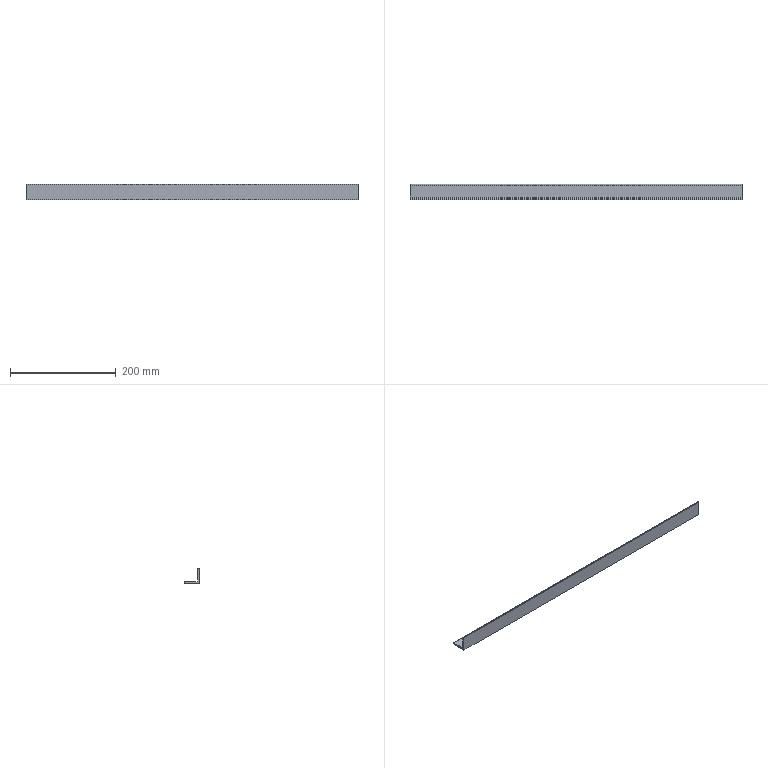Part | NX | features BREP 1 | 1 solid | 11 faces | box 627.062 x 28.575 x 28.575 mm | volume 107121 mm3 | plane 8 | cylinder 3 | commonest cylinder face diameters 3.175 x3
STEP:
#1=CARTESIAN_POINT('',(-313.531,-1.587,25.4));
#2=VERTEX_POINT('',#1);
#3=CARTESIAN_POINT('',(-313.531,0.,23.812));
#4=VERTEX_POINT('',#3);
#5=CARTESIAN_POINT('',(-313.531,-1.587,23.812));
#6=DIRECTION('',(-1.,0.,0.));
#7=DIRECTION('',(0.,0.,1.));
#8=AXIS2_PLACEMENT_3D('',#5,#6,#7);
#9=CIRCLE('',#8,1.587);
#10=EDGE_CURVE('',#2,#4,#9,.T.);
#11=ORIENTED_EDGE('',*,*,#10,.T.);
#12=CARTESIAN_POINT('',(-313.531,0.,1.587));
#13=VERTEX_POINT('',#12);
#14=CARTESIAN_POINT('',(-313.531,0.,1.587));
#15=DIRECTION('',(0.,0.,1.));
#16=VECTOR('',#15,1000.);
#17=LINE('',#14,#16);
#18=EDGE_CURVE('',#13,#4,#17,.T.);
#19=ORIENTED_EDGE('',*,*,#18,.F.);
#20=CARTESIAN_POINT('',(-313.531,1.587,0.));
#21=VERTEX_POINT('',#20);
#22=CARTESIAN_POINT('',(-313.531,1.587,1.587));
#23=DIRECTION('',(1.,0.,0.));
#24=DIRECTION('',(0.,-1.,0.));
#25=AXIS2_PLACEMENT_3D('',#22,#23,#24);
#26=CIRCLE('',#25,1.587);
#27=EDGE_CURVE('',#13,#21,#26,.T.);
#28=ORIENTED_EDGE('',*,*,#27,.T.);
#29=CARTESIAN_POINT('',(-313.531,23.812,0.));
#30=VERTEX_POINT('',#29);
#31=CARTESIAN_POINT('',(-313.531,23.812,0.));
#32=DIRECTION('',(0.,-1.,0.));
#33=VECTOR('',#32,1000.);
#34=LINE('',#31,#33);
#35=EDGE_CURVE('',#30,#21,#34,.T.);
#36=ORIENTED_EDGE('',*,*,#35,.F.);
#37=CARTESIAN_POINT('',(-313.531,25.4,-1.587));
#38=VERTEX_POINT('',#37);
#39=CARTESIAN_POINT('',(-313.531,23.812,-1.587));
#40=DIRECTION('',(-1.,0.,0.));
#41=DIRECTION('',(0.,0.,1.));
#42=AXIS2_PLACEMENT_3D('',#39,#40,#41);
#43=CIRCLE('',#42,1.587);
#44=EDGE_CURVE('',#30,#38,#43,.T.);
#45=ORIENTED_EDGE('',*,*,#44,.T.);
#46=CARTESIAN_POINT('',(-313.531,25.4,-3.175));
#47=VERTEX_POINT('',#46);
#48=CARTESIAN_POINT('',(-313.531,25.4,-3.175));
#49=DIRECTION('',(0.,0.,1.));
#50=VECTOR('',#49,1000.);
#51=LINE('',#48,#50);
#52=EDGE_CURVE('',#47,#38,#51,.T.);
#53=ORIENTED_EDGE('',*,*,#52,.F.);
#54=CARTESIAN_POINT('',(-313.531,-3.175,-3.175));
#55=VERTEX_POINT('',#54);
#56=CARTESIAN_POINT('',(-313.531,-3.175,-3.175));
#57=DIRECTION('',(0.,1.,0.));
#58=VECTOR('',#57,1000.);
#59=LINE('',#56,#58);
#60=EDGE_CURVE('',#55,#47,#59,.T.);
#61=ORIENTED_EDGE('',*,*,#60,.F.);
#62=CARTESIAN_POINT('',(-313.531,-3.175,25.4));
#63=VERTEX_POINT('',#62);
#64=CARTESIAN_POINT('',(-313.531,-3.175,25.4));
#65=DIRECTION('',(0.,0.,-1.));
#66=VECTOR('',#65,1000.);
#67=LINE('',#64,#66);
#68=EDGE_CURVE('',#63,#55,#67,.T.);
#69=ORIENTED_EDGE('',*,*,#68,.F.);
#70=CARTESIAN_POINT('',(-313.531,-1.587,25.4));
#71=DIRECTION('',(0.,-1.,0.));
#72=VECTOR('',#71,1000.);
#73=LINE('',#70,#72);
#74=EDGE_CURVE('',#2,#63,#73,.T.);
#75=ORIENTED_EDGE('',*,*,#74,.F.);
#76=EDGE_LOOP('',(#11,#19,#28,#36,#45,#53,#61,#69,#75));
#77=FACE_BOUND('',#76,.T.);
#78=CARTESIAN_POINT('',(-313.531,0.,0.));
#79=DIRECTION('',(1.,0.,0.));
#80=DIRECTION('',(0.,1.,0.));
#81=AXIS2_PLACEMENT_3D('',#78,#79,#80);
#82=PLANE('',#81);
#83=ADVANCED_FACE('',(#77),#82,.F.);
#84=CARTESIAN_POINT('',(313.531,-3.175,25.4));
#85=VERTEX_POINT('',#84);
#86=CARTESIAN_POINT('',(-313.531,-3.175,25.4));
#87=DIRECTION('',(1.,0.,0.));
#88=VECTOR('',#87,1000.);
#89=LINE('',#86,#88);
#90=EDGE_CURVE('',#63,#85,#89,.T.);
#91=ORIENTED_EDGE('',*,*,#90,.T.);
#92=CARTESIAN_POINT('',(313.531,-1.587,25.4));
#93=VERTEX_POINT('',#92);
#94=CARTESIAN_POINT('',(313.531,-1.587,25.4));
#95=DIRECTION('',(0.,-1.,0.));
#96=VECTOR('',#95,1000.);
#97=LINE('',#94,#96);
#98=EDGE_CURVE('',#93,#85,#97,.T.);
#99=ORIENTED_EDGE('',*,*,#98,.F.);
#100=CARTESIAN_POINT('',(313.531,-1.587,25.4));
#101=DIRECTION('',(-1.,0.,0.));
#102=VECTOR('',#101,1000.);
#103=LINE('',#100,#102);
#104=EDGE_CURVE('',#93,#2,#103,.T.);
#105=ORIENTED_EDGE('',*,*,#104,.T.);
#106=ORIENTED_EDGE('',*,*,#74,.T.);
#107=EDGE_LOOP('',(#91,#99,#105,#106));
#108=FACE_BOUND('',#107,.T.);
#109=CARTESIAN_POINT('',(-313.531,0.,25.4));
#110=DIRECTION('',(0.,0.,1.));
#111=DIRECTION('',(1.,0.,0.));
#112=AXIS2_PLACEMENT_3D('',#109,#110,#111);
#113=PLANE('',#112);
#114=ADVANCED_FACE('',(#108),#113,.T.);
#115=CARTESIAN_POINT('',(313.531,0.,23.812));
#116=VERTEX_POINT('',#115);
#117=CARTESIAN_POINT('',(313.531,-1.587,23.812));
#118=DIRECTION('',(1.,0.,0.));
#119=DIRECTION('',(0.,1.,0.));
#120=AXIS2_PLACEMENT_3D('',#117,#118,#119);
#121=CIRCLE('',#120,1.587);
#122=EDGE_CURVE('',#116,#93,#121,.T.);
#123=ORIENTED_EDGE('',*,*,#122,.F.);
#124=CARTESIAN_POINT('',(313.531,0.,23.812));
#125=DIRECTION('',(-1.,0.,0.));
#126=VECTOR('',#125,1000.);
#127=LINE('',#124,#126);
#128=EDGE_CURVE('',#116,#4,#127,.T.);
#129=ORIENTED_EDGE('',*,*,#128,.T.);
#130=ORIENTED_EDGE('',*,*,#10,.F.);
#131=ORIENTED_EDGE('',*,*,#104,.F.);
#132=EDGE_LOOP('',(#123,#129,#130,#131));
#133=FACE_BOUND('',#132,.T.);
#134=CARTESIAN_POINT('',(314.514,-1.587,23.812));
#135=DIRECTION('',(-1.,0.,0.));
#136=DIRECTION('',(0.,0.,1.));
#137=AXIS2_PLACEMENT_3D('',#134,#135,#136);
#138=CYLINDRICAL_SURFACE('',#137,1.587);
#139=ADVANCED_FACE('',(#133),#138,.T.);
#140=CARTESIAN_POINT('',(313.531,0.,1.587));
#141=VERTEX_POINT('',#140);
#142=CARTESIAN_POINT('',(313.531,0.,1.587));
#143=DIRECTION('',(0.,0.,1.));
#144=VECTOR('',#143,1000.);
#145=LINE('',#142,#144);
#146=EDGE_CURVE('',#141,#116,#145,.T.);
#147=ORIENTED_EDGE('',*,*,#146,.F.);
#148=CARTESIAN_POINT('',(-313.531,0.,1.587));
#149=DIRECTION('',(1.,0.,0.));
#150=VECTOR('',#149,1000.);
#151=LINE('',#148,#150);
#152=EDGE_CURVE('',#13,#141,#151,.T.);
#153=ORIENTED_EDGE('',*,*,#152,.F.);
#154=ORIENTED_EDGE('',*,*,#18,.T.);
#155=ORIENTED_EDGE('',*,*,#128,.F.);
#156=EDGE_LOOP('',(#147,#153,#154,#155));
#157=FACE_BOUND('',#156,.T.);
#158=CARTESIAN_POINT('',(-313.531,0.,0.));
#159=DIRECTION('',(0.,1.,0.));
#160=DIRECTION('',(1.,0.,0.));
#161=AXIS2_PLACEMENT_3D('',#158,#159,#160);
#162=PLANE('',#161);
#163=ADVANCED_FACE('',(#157),#162,.T.);
#164=CARTESIAN_POINT('',(313.531,1.587,0.));
#165=VERTEX_POINT('',#164);
#166=CARTESIAN_POINT('',(313.531,1.587,1.587));
#167=DIRECTION('',(-1.,0.,0.));
#168=DIRECTION('',(0.,0.,-1.));
#169=AXIS2_PLACEMENT_3D('',#166,#167,#168);
#170=CIRCLE('',#169,1.587);
#171=EDGE_CURVE('',#165,#141,#170,.T.);
#172=ORIENTED_EDGE('',*,*,#171,.F.);
#173=CARTESIAN_POINT('',(-313.531,1.587,0.));
#174=DIRECTION('',(1.,0.,0.));
#175=VECTOR('',#174,1000.);
#176=LINE('',#173,#175);
#177=EDGE_CURVE('',#21,#165,#176,.T.);
#178=ORIENTED_EDGE('',*,*,#177,.F.);
#179=ORIENTED_EDGE('',*,*,#27,.F.);
#180=ORIENTED_EDGE('',*,*,#152,.T.);
#181=EDGE_LOOP('',(#172,#178,#179,#180));
#182=FACE_BOUND('',#181,.T.);
#183=CARTESIAN_POINT('',(-314.371,1.587,1.587));
#184=DIRECTION('',(1.,0.,0.));
#185=DIRECTION('',(0.,-1.,0.));
#186=AXIS2_PLACEMENT_3D('',#183,#184,#185);
#187=CYLINDRICAL_SURFACE('',#186,1.587);
#188=ADVANCED_FACE('',(#182),#187,.F.);
#189=ORIENTED_EDGE('',*,*,#35,.T.);
#190=ORIENTED_EDGE('',*,*,#177,.T.);
#191=CARTESIAN_POINT('',(313.531,23.812,0.));
#192=VERTEX_POINT('',#191);
#193=CARTESIAN_POINT('',(313.531,23.812,0.));
#194=DIRECTION('',(0.,-1.,0.));
#195=VECTOR('',#194,1000.);
#196=LINE('',#193,#195);
#197=EDGE_CURVE('',#192,#165,#196,.T.);
#198=ORIENTED_EDGE('',*,*,#197,.F.);
#199=CARTESIAN_POINT('',(313.531,23.812,0.));
#200=DIRECTION('',(-1.,0.,0.));
#201=VECTOR('',#200,1000.);
#202=LINE('',#199,#201);
#203=EDGE_CURVE('',#192,#30,#202,.T.);
#204=ORIENTED_EDGE('',*,*,#203,.T.);
#205=EDGE_LOOP('',(#189,#190,#198,#204));
#206=FACE_BOUND('',#205,.T.);
#207=CARTESIAN_POINT('',(-313.531,25.4,0.));
#208=DIRECTION('',(0.,0.,1.));
#209=DIRECTION('',(1.,0.,0.));
#210=AXIS2_PLACEMENT_3D('',#207,#208,#209);
#211=PLANE('',#210);
#212=ADVANCED_FACE('',(#206),#211,.T.);
#213=CARTESIAN_POINT('',(313.531,25.4,-1.587));
#214=VERTEX_POINT('',#213);
#215=CARTESIAN_POINT('',(313.531,23.812,-1.587));
#216=DIRECTION('',(1.,0.,0.));
#217=DIRECTION('',(0.,1.,0.));
#218=AXIS2_PLACEMENT_3D('',#215,#216,#217);
#219=CIRCLE('',#218,1.587);
#220=EDGE_CURVE('',#214,#192,#219,.T.);
#221=ORIENTED_EDGE('',*,*,#220,.F.);
#222=CARTESIAN_POINT('',(313.531,25.4,-1.587));
#223=DIRECTION('',(-1.,0.,0.));
#224=VECTOR('',#223,1000.);
#225=LINE('',#222,#224);
#226=EDGE_CURVE('',#214,#38,#225,.T.);
#227=ORIENTED_EDGE('',*,*,#226,.T.);
#228=ORIENTED_EDGE('',*,*,#44,.F.);
#229=ORIENTED_EDGE('',*,*,#203,.F.);
#230=EDGE_LOOP('',(#221,#227,#228,#229));
#231=FACE_BOUND('',#230,.T.);
#232=CARTESIAN_POINT('',(314.514,23.812,-1.587));
#233=DIRECTION('',(-1.,0.,0.));
#234=DIRECTION('',(0.,0.,1.));
#235=AXIS2_PLACEMENT_3D('',#232,#233,#234);
#236=CYLINDRICAL_SURFACE('',#235,1.587);
#237=ADVANCED_FACE('',(#231),#236,.T.);
#238=ORIENTED_EDGE('',*,*,#226,.F.);
#239=CARTESIAN_POINT('',(313.531,25.4,-3.175));
#240=VERTEX_POINT('',#239);
#241=CARTESIAN_POINT('',(313.531,25.4,-3.175));
#242=DIRECTION('',(0.,0.,1.));
#243=VECTOR('',#242,1000.);
#244=LINE('',#241,#243);
#245=EDGE_CURVE('',#240,#214,#244,.T.);
#246=ORIENTED_EDGE('',*,*,#245,.F.);
#247=CARTESIAN_POINT('',(-313.531,25.4,-3.175));
#248=DIRECTION('',(1.,0.,0.));
#249=VECTOR('',#248,1000.);
#250=LINE('',#247,#249);
#251=EDGE_CURVE('',#47,#240,#250,.T.);
#252=ORIENTED_EDGE('',*,*,#251,.F.);
#253=ORIENTED_EDGE('',*,*,#52,.T.);
#254=EDGE_LOOP('',(#238,#246,#252,#253));
#255=FACE_BOUND('',#254,.T.);
#256=CARTESIAN_POINT('',(-313.531,25.4,-3.175));
#257=DIRECTION('',(0.,1.,0.));
#258=DIRECTION('',(1.,0.,0.));
#259=AXIS2_PLACEMENT_3D('',#256,#257,#258);
#260=PLANE('',#259);
#261=ADVANCED_FACE('',(#255),#260,.T.);
#262=ORIENTED_EDGE('',*,*,#251,.T.);
#263=CARTESIAN_POINT('',(313.531,-3.175,-3.175));
#264=VERTEX_POINT('',#263);
#265=CARTESIAN_POINT('',(313.531,-3.175,-3.175));
#266=DIRECTION('',(0.,1.,0.));
#267=VECTOR('',#266,1000.);
#268=LINE('',#265,#267);
#269=EDGE_CURVE('',#264,#240,#268,.T.);
#270=ORIENTED_EDGE('',*,*,#269,.F.);
#271=CARTESIAN_POINT('',(-313.531,-3.175,-3.175));
#272=DIRECTION('',(1.,0.,0.));
#273=VECTOR('',#272,1000.);
#274=LINE('',#271,#273);
#275=EDGE_CURVE('',#55,#264,#274,.T.);
#276=ORIENTED_EDGE('',*,*,#275,.F.);
#277=ORIENTED_EDGE('',*,*,#60,.T.);
#278=EDGE_LOOP('',(#262,#270,#276,#277));
#279=FACE_BOUND('',#278,.T.);
#280=CARTESIAN_POINT('',(-313.531,-3.175,-3.175));
#281=DIRECTION('',(0.,0.,-1.));
#282=DIRECTION('',(0.,-1.,0.));
#283=AXIS2_PLACEMENT_3D('',#280,#281,#282);
#284=PLANE('',#283);
#285=ADVANCED_FACE('',(#279),#284,.T.);
#286=ORIENTED_EDGE('',*,*,#275,.T.);
#287=CARTESIAN_POINT('',(313.531,-3.175,25.4));
#288=DIRECTION('',(0.,0.,-1.));
#289=VECTOR('',#288,1000.);
#290=LINE('',#287,#289);
#291=EDGE_CURVE('',#85,#264,#290,.T.);
#292=ORIENTED_EDGE('',*,*,#291,.F.);
#293=ORIENTED_EDGE('',*,*,#90,.F.);
#294=ORIENTED_EDGE('',*,*,#68,.T.);
#295=EDGE_LOOP('',(#286,#292,#293,#294));
#296=FACE_BOUND('',#295,.T.);
#297=CARTESIAN_POINT('',(-313.531,-3.175,25.4));
#298=DIRECTION('',(0.,-1.,0.));
#299=DIRECTION('',(0.,0.,-1.));
#300=AXIS2_PLACEMENT_3D('',#297,#298,#299);
#301=PLANE('',#300);
#302=ADVANCED_FACE('',(#296),#301,.T.);
#303=ORIENTED_EDGE('',*,*,#291,.T.);
#304=ORIENTED_EDGE('',*,*,#269,.T.);
#305=ORIENTED_EDGE('',*,*,#245,.T.);
#306=ORIENTED_EDGE('',*,*,#220,.T.);
#307=ORIENTED_EDGE('',*,*,#197,.T.);
#308=ORIENTED_EDGE('',*,*,#171,.T.);
#309=ORIENTED_EDGE('',*,*,#146,.T.);
#310=ORIENTED_EDGE('',*,*,#122,.T.);
#311=ORIENTED_EDGE('',*,*,#98,.T.);
#312=EDGE_LOOP('',(#303,#304,#305,#306,#307,#308,#309,#310,#311));
#313=FACE_BOUND('',#312,.T.);
#314=CARTESIAN_POINT('',(313.531,0.,0.));
#315=DIRECTION('',(1.,0.,0.));
#316=DIRECTION('',(0.,1.,0.));
#317=AXIS2_PLACEMENT_3D('',#314,#315,#316);
#318=PLANE('',#317);
#319=ADVANCED_FACE('',(#313),#318,.T.);
#320=CLOSED_SHELL('',(#83,#114,#139,#163,#188,#212,#237,#261,#285,#302,#319));
#321=MANIFOLD_SOLID_BREP('',#320);
#322=(LENGTH_UNIT()NAMED_UNIT(*)SI_UNIT(.MILLI.,.METRE.));
#323=UNCERTAINTY_MEASURE_WITH_UNIT(LENGTH_MEASURE(0.00001),#322,'','');
#324=(NAMED_UNIT(*)PLANE_ANGLE_UNIT()SI_UNIT($,.RADIAN.));
#325=(NAMED_UNIT(*)SI_UNIT($,.STERADIAN.)SOLID_ANGLE_UNIT());
#326=(GEOMETRIC_REPRESENTATION_CONTEXT(3)GLOBAL_UNCERTAINTY_ASSIGNED_CONTEXT((#323))GLOBAL_UNIT_ASSIGNED_CONTEXT((#322,#324,#325))REPRESENTATION_CONTEXT('',''));
#327=ADVANCED_BREP_SHAPE_REPRESENTATION('',(#321),#326);